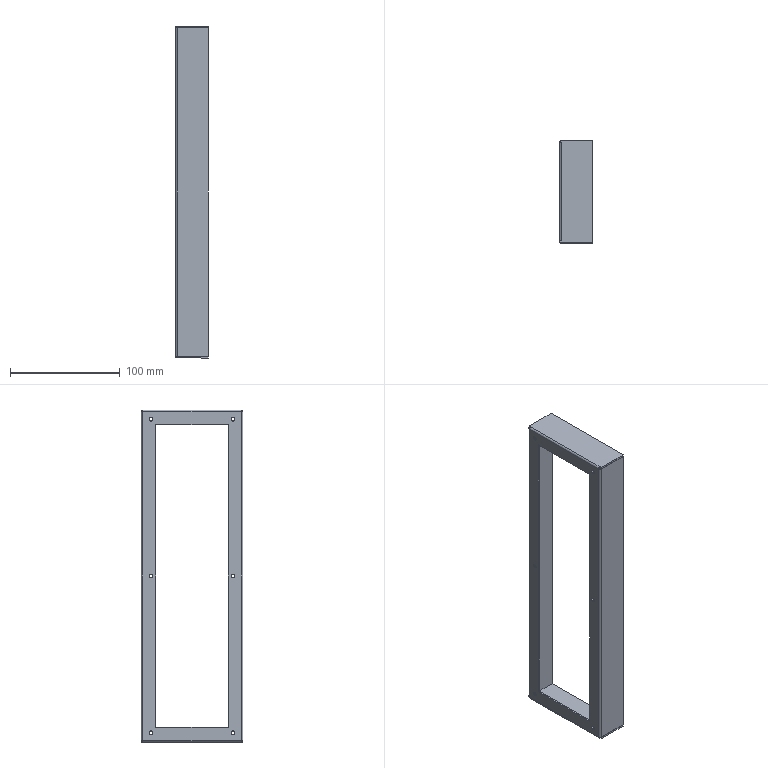Part | SolidWorks | features EdgeFlange 2, FlatPattern 1, HoleWzd 1, ICE 1, SMBaseFlange 1, SheetMetal 1 | 1 solid | 58 faces | box 30 x 93 x 303 mm | volume 47939 mm3 | plane 38 | cylinder 20 | commonest cylinder face diameters 3.3 x12 0.4 x4 3.4 x4